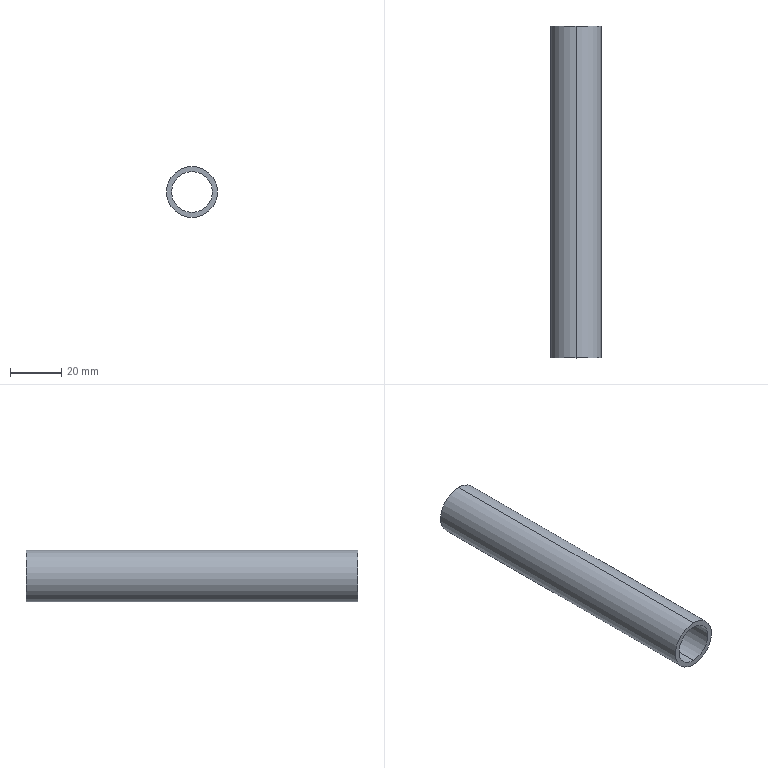Part | SolidWorks | features Extrusion 1 | 1 solid | 6 faces | box 20 x 130 x 20 mm | volume 14703 mm3 | cylinder 4 | plane 2 | commonest cylinder face diameters 16 x2 20 x2
STEP:
#1=CARTESIAN_POINT('',(0.,130.,-8.));
#2=VERTEX_POINT('',#1);
#3=CARTESIAN_POINT('',(0.,130.,8.));
#4=VERTEX_POINT('',#3);
#5=CARTESIAN_POINT('',(0.,130.,0.));
#6=DIRECTION('',(0.,1.,0.));
#7=DIRECTION('',(0.,0.,1.));
#8=AXIS2_PLACEMENT_3D('',#5,#6,#7);
#9=CIRCLE('',#8,8.);
#10=EDGE_CURVE('',#2,#4,#9,.T.);
#11=ORIENTED_EDGE('',*,*,#10,.T.);
#12=CARTESIAN_POINT('',(0.,0.,8.));
#13=VERTEX_POINT('',#12);
#14=CARTESIAN_POINT('',(0.,130.,8.));
#15=DIRECTION('',(0.,-1.,0.));
#16=VECTOR('',#15,1000.);
#17=LINE('',#14,#16);
#18=EDGE_CURVE('',#4,#13,#17,.T.);
#19=ORIENTED_EDGE('',*,*,#18,.T.);
#20=CARTESIAN_POINT('',(0.,0.,-8.));
#21=VERTEX_POINT('',#20);
#22=CARTESIAN_POINT('',(0.,0.,0.));
#23=DIRECTION('',(0.,1.,0.));
#24=DIRECTION('',(0.,0.,1.));
#25=AXIS2_PLACEMENT_3D('',#22,#23,#24);
#26=CIRCLE('',#25,8.);
#27=EDGE_CURVE('',#21,#13,#26,.T.);
#28=ORIENTED_EDGE('',*,*,#27,.F.);
#29=CARTESIAN_POINT('',(0.,130.,-8.));
#30=DIRECTION('',(0.,-1.,0.));
#31=VECTOR('',#30,1000.);
#32=LINE('',#29,#31);
#33=EDGE_CURVE('',#2,#21,#32,.T.);
#34=ORIENTED_EDGE('',*,*,#33,.F.);
#35=EDGE_LOOP('',(#11,#19,#28,#34));
#36=FACE_OUTER_BOUND('',#35,.T.);
#37=CARTESIAN_POINT('',(0.,130.,0.));
#38=DIRECTION('',(0.,-1.,0.));
#39=DIRECTION('',(0.,0.,-1.));
#40=AXIS2_PLACEMENT_3D('',#37,#38,#39);
#41=CYLINDRICAL_SURFACE('',#40,8.);
#42=ADVANCED_FACE('',(#36),#41,.F.);
#43=CARTESIAN_POINT('',(0.,130.,10.));
#44=VERTEX_POINT('',#43);
#45=CARTESIAN_POINT('',(0.,130.,-10.));
#46=VERTEX_POINT('',#45);
#47=CARTESIAN_POINT('',(0.,130.,0.));
#48=DIRECTION('',(0.,1.,0.));
#49=DIRECTION('',(0.,0.,1.));
#50=AXIS2_PLACEMENT_3D('',#47,#48,#49);
#51=CIRCLE('',#50,10.);
#52=EDGE_CURVE('',#44,#46,#51,.T.);
#53=ORIENTED_EDGE('',*,*,#52,.F.);
#54=CARTESIAN_POINT('',(0.,0.,10.));
#55=VERTEX_POINT('',#54);
#56=CARTESIAN_POINT('',(0.,130.,10.));
#57=DIRECTION('',(0.,-1.,0.));
#58=VECTOR('',#57,1000.);
#59=LINE('',#56,#58);
#60=EDGE_CURVE('',#44,#55,#59,.T.);
#61=ORIENTED_EDGE('',*,*,#60,.T.);
#62=CARTESIAN_POINT('',(0.,0.,-10.));
#63=VERTEX_POINT('',#62);
#64=CARTESIAN_POINT('',(0.,0.,0.));
#65=DIRECTION('',(0.,1.,0.));
#66=DIRECTION('',(0.,0.,1.));
#67=AXIS2_PLACEMENT_3D('',#64,#65,#66);
#68=CIRCLE('',#67,10.);
#69=EDGE_CURVE('',#55,#63,#68,.T.);
#70=ORIENTED_EDGE('',*,*,#69,.T.);
#71=CARTESIAN_POINT('',(0.,130.,-10.));
#72=DIRECTION('',(0.,-1.,0.));
#73=VECTOR('',#72,1000.);
#74=LINE('',#71,#73);
#75=EDGE_CURVE('',#46,#63,#74,.T.);
#76=ORIENTED_EDGE('',*,*,#75,.F.);
#77=EDGE_LOOP('',(#53,#61,#70,#76));
#78=FACE_OUTER_BOUND('',#77,.T.);
#79=CARTESIAN_POINT('',(0.,130.,0.));
#80=DIRECTION('',(0.,-1.,0.));
#81=DIRECTION('',(0.,0.,-1.));
#82=AXIS2_PLACEMENT_3D('',#79,#80,#81);
#83=CYLINDRICAL_SURFACE('',#82,10.);
#84=ADVANCED_FACE('',(#78),#83,.T.);
#85=CARTESIAN_POINT('',(0.,130.,0.));
#86=DIRECTION('',(0.,1.,0.));
#87=DIRECTION('',(0.,0.,1.));
#88=AXIS2_PLACEMENT_3D('',#85,#86,#87);
#89=CIRCLE('',#88,10.);
#90=EDGE_CURVE('',#46,#44,#89,.T.);
#91=ORIENTED_EDGE('',*,*,#90,.T.);
#92=ORIENTED_EDGE('',*,*,#52,.T.);
#93=EDGE_LOOP('',(#91,#92));
#94=FACE_OUTER_BOUND('',#93,.T.);
#95=ORIENTED_EDGE('',*,*,#10,.F.);
#96=CARTESIAN_POINT('',(0.,130.,0.));
#97=DIRECTION('',(0.,1.,0.));
#98=DIRECTION('',(0.,0.,1.));
#99=AXIS2_PLACEMENT_3D('',#96,#97,#98);
#100=CIRCLE('',#99,8.);
#101=EDGE_CURVE('',#4,#2,#100,.T.);
#102=ORIENTED_EDGE('',*,*,#101,.F.);
#103=EDGE_LOOP('',(#95,#102));
#104=FACE_BOUND('',#103,.T.);
#105=CARTESIAN_POINT('',(0.,130.,0.));
#106=DIRECTION('',(0.,1.,0.));
#107=DIRECTION('',(0.,0.,1.));
#108=AXIS2_PLACEMENT_3D('',#105,#106,#107);
#109=PLANE('',#108);
#110=ADVANCED_FACE('',(#94,#104),#109,.T.);
#111=CARTESIAN_POINT('',(0.,0.,0.));
#112=DIRECTION('',(0.,1.,0.));
#113=DIRECTION('',(0.,0.,1.));
#114=AXIS2_PLACEMENT_3D('',#111,#112,#113);
#115=CIRCLE('',#114,10.);
#116=EDGE_CURVE('',#63,#55,#115,.T.);
#117=ORIENTED_EDGE('',*,*,#116,.F.);
#118=ORIENTED_EDGE('',*,*,#69,.F.);
#119=EDGE_LOOP('',(#117,#118));
#120=FACE_OUTER_BOUND('',#119,.T.);
#121=ORIENTED_EDGE('',*,*,#27,.T.);
#122=CARTESIAN_POINT('',(0.,0.,0.));
#123=DIRECTION('',(0.,1.,0.));
#124=DIRECTION('',(0.,0.,1.));
#125=AXIS2_PLACEMENT_3D('',#122,#123,#124);
#126=CIRCLE('',#125,8.);
#127=EDGE_CURVE('',#13,#21,#126,.T.);
#128=ORIENTED_EDGE('',*,*,#127,.T.);
#129=EDGE_LOOP('',(#121,#128));
#130=FACE_BOUND('',#129,.T.);
#131=CARTESIAN_POINT('',(0.,0.,0.));
#132=DIRECTION('',(0.,1.,0.));
#133=DIRECTION('',(0.,0.,1.));
#134=AXIS2_PLACEMENT_3D('',#131,#132,#133);
#135=PLANE('',#134);
#136=ADVANCED_FACE('',(#120,#130),#135,.F.);
#137=ORIENTED_EDGE('',*,*,#60,.F.);
#138=ORIENTED_EDGE('',*,*,#90,.F.);
#139=ORIENTED_EDGE('',*,*,#75,.T.);
#140=ORIENTED_EDGE('',*,*,#116,.T.);
#141=EDGE_LOOP('',(#137,#138,#139,#140));
#142=FACE_OUTER_BOUND('',#141,.T.);
#143=CARTESIAN_POINT('',(0.,130.,0.));
#144=DIRECTION('',(0.,-1.,0.));
#145=DIRECTION('',(0.,0.,-1.));
#146=AXIS2_PLACEMENT_3D('',#143,#144,#145);
#147=CYLINDRICAL_SURFACE('',#146,10.);
#148=ADVANCED_FACE('',(#142),#147,.T.);
#149=ORIENTED_EDGE('',*,*,#18,.F.);
#150=ORIENTED_EDGE('',*,*,#101,.T.);
#151=ORIENTED_EDGE('',*,*,#33,.T.);
#152=ORIENTED_EDGE('',*,*,#127,.F.);
#153=EDGE_LOOP('',(#149,#150,#151,#152));
#154=FACE_OUTER_BOUND('',#153,.T.);
#155=CARTESIAN_POINT('',(0.,130.,0.));
#156=DIRECTION('',(0.,-1.,0.));
#157=DIRECTION('',(0.,0.,-1.));
#158=AXIS2_PLACEMENT_3D('',#155,#156,#157);
#159=CYLINDRICAL_SURFACE('',#158,8.);
#160=ADVANCED_FACE('',(#154),#159,.F.);
#161=CLOSED_SHELL('',(#42,#84,#110,#136,#148,#160));
#162=MANIFOLD_SOLID_BREP('',#161);
#163=CARTESIAN_POINT('',(0.,0.,0.));
#164=DIRECTION('',(0.,0.,1.));
#165=DIRECTION('',(1.,0.,0.));
#166=AXIS2_PLACEMENT_3D('',#163,#164,#165);
#167=(LENGTH_UNIT()NAMED_UNIT(*)SI_UNIT(.MILLI.,.METRE.));
#168=UNCERTAINTY_MEASURE_WITH_UNIT(LENGTH_MEASURE(0.00001),#167,'','');
#169=(NAMED_UNIT(*)PLANE_ANGLE_UNIT()SI_UNIT($,.RADIAN.));
#170=(NAMED_UNIT(*)SI_UNIT($,.STERADIAN.)SOLID_ANGLE_UNIT());
#171=(GEOMETRIC_REPRESENTATION_CONTEXT(3)GLOBAL_UNCERTAINTY_ASSIGNED_CONTEXT((#168))GLOBAL_UNIT_ASSIGNED_CONTEXT((#167,#169,#170))REPRESENTATION_CONTEXT('',''));
#172=ADVANCED_BREP_SHAPE_REPRESENTATION('',(#162,#166),#171);